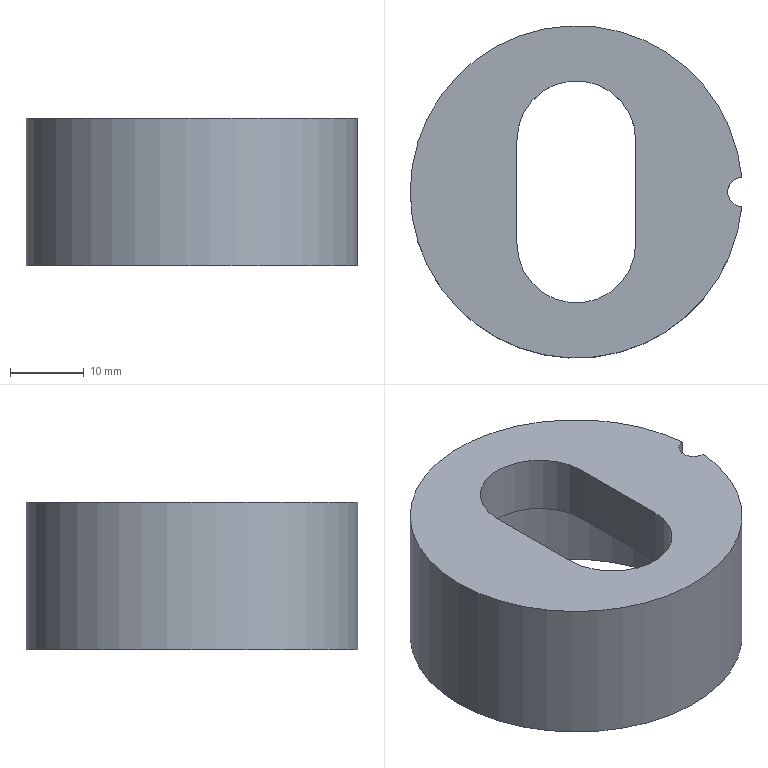Part | NX | features solid 2 | 1 solid | 10 faces | box 44.911 x 45 x 20 mm | volume 16039 mm3 | cylinder 5 | plane 5 | commonest cylinder face diameters 16.1 x2 4 x1 36 x1 45 x1
STEP:
#1=CARTESIAN_POINT('',(334.41,166.18,-1.322));
#2=VERTEX_POINT('',#1);
#3=CARTESIAN_POINT('',(334.41,166.18,18.678));
#4=VERTEX_POINT('',#3);
#5=CARTESIAN_POINT('',(334.41,166.18,8.678));
#6=DIRECTION('',(0.,0.,1.));
#7=VECTOR('',#6,1000.);
#8=LINE('',#5,#7);
#9=EDGE_CURVE('',#2,#4,#8,.T.);
#10=ORIENTED_EDGE('',*,*,#9,.F.);
#11=CARTESIAN_POINT('',(334.41,162.184,-1.322));
#12=VERTEX_POINT('',#11);
#13=CARTESIAN_POINT('',(311.999,164.182,-1.322));
#14=DIRECTION('',(0.,0.,1.));
#15=DIRECTION('',(1.,0.,0.));
#16=AXIS2_PLACEMENT_3D('',#13,#14,#15);
#17=CIRCLE('',#16,22.5);
#18=EDGE_CURVE('',#2,#12,#17,.T.);
#19=ORIENTED_EDGE('',*,*,#18,.T.);
#20=CARTESIAN_POINT('',(334.41,162.184,18.678));
#21=VERTEX_POINT('',#20);
#22=CARTESIAN_POINT('',(334.41,162.184,8.678));
#23=DIRECTION('',(0.,0.,1.));
#24=VECTOR('',#23,1000.);
#25=LINE('',#22,#24);
#26=EDGE_CURVE('',#21,#12,#25,.F.);
#27=ORIENTED_EDGE('',*,*,#26,.F.);
#28=CARTESIAN_POINT('',(311.999,164.182,18.678));
#29=DIRECTION('',(0.,0.,1.));
#30=DIRECTION('',(1.,0.,0.));
#31=AXIS2_PLACEMENT_3D('',#28,#29,#30);
#32=CIRCLE('',#31,22.5);
#33=EDGE_CURVE('',#4,#21,#32,.T.);
#34=ORIENTED_EDGE('',*,*,#33,.F.);
#35=EDGE_LOOP('',(#10,#19,#27,#34));
#36=FACE_BOUND('',#35,.T.);
#37=CARTESIAN_POINT('',(311.999,164.182,-1.322));
#38=DIRECTION('',(0.,0.,1.));
#39=DIRECTION('',(1.,0.,0.));
#40=AXIS2_PLACEMENT_3D('',#37,#38,#39);
#41=CYLINDRICAL_SURFACE('',#40,22.5);
#42=ADVANCED_FACE('',(#36),#41,.T.);
#43=CARTESIAN_POINT('',(329.999,164.182,-1.322));
#44=VERTEX_POINT('',#43);
#45=CARTESIAN_POINT('',(311.999,164.182,-1.322));
#46=DIRECTION('',(0.,0.,1.));
#47=DIRECTION('',(1.,0.,0.));
#48=AXIS2_PLACEMENT_3D('',#45,#46,#47);
#49=CIRCLE('',#48,18.);
#50=EDGE_CURVE('',#44,#44,#49,.T.);
#51=ORIENTED_EDGE('',*,*,#50,.T.);
#52=EDGE_LOOP('',(#51));
#53=FACE_BOUND('',#52,.T.);
#54=ORIENTED_EDGE('',*,*,#18,.F.);
#55=CARTESIAN_POINT('',(334.499,164.182,-1.322));
#56=DIRECTION('',(0.,0.,1.));
#57=DIRECTION('',(1.,0.,0.));
#58=AXIS2_PLACEMENT_3D('',#55,#56,#57);
#59=CIRCLE('',#58,2.);
#60=EDGE_CURVE('',#2,#12,#59,.T.);
#61=ORIENTED_EDGE('',*,*,#60,.T.);
#62=EDGE_LOOP('',(#54,#61));
#63=FACE_BOUND('',#62,.T.);
#64=CARTESIAN_POINT('',(311.999,164.182,-1.322));
#65=DIRECTION('',(0.,0.,1.));
#66=DIRECTION('',(1.,0.,0.));
#67=AXIS2_PLACEMENT_3D('',#64,#65,#66);
#68=PLANE('',#67);
#69=ADVANCED_FACE('',(#53,#63),#68,.F.);
#70=CARTESIAN_POINT('',(303.949,171.182,18.678));
#71=VERTEX_POINT('',#70);
#72=CARTESIAN_POINT('',(303.949,157.182,18.678));
#73=VERTEX_POINT('',#72);
#74=CARTESIAN_POINT('',(303.949,171.182,18.678));
#75=DIRECTION('',(0.,-1.,0.));
#76=VECTOR('',#75,1000.);
#77=LINE('',#74,#76);
#78=EDGE_CURVE('',#71,#73,#77,.T.);
#79=ORIENTED_EDGE('',*,*,#78,.F.);
#80=CARTESIAN_POINT('',(320.049,171.182,18.678));
#81=VERTEX_POINT('',#80);
#82=CARTESIAN_POINT('',(311.999,171.182,18.678));
#83=DIRECTION('',(0.,0.,1.));
#84=DIRECTION('',(1.,0.,0.));
#85=AXIS2_PLACEMENT_3D('',#82,#83,#84);
#86=CIRCLE('',#85,8.05);
#87=EDGE_CURVE('',#81,#71,#86,.T.);
#88=ORIENTED_EDGE('',*,*,#87,.F.);
#89=CARTESIAN_POINT('',(320.049,157.182,18.678));
#90=VERTEX_POINT('',#89);
#91=CARTESIAN_POINT('',(320.049,171.182,18.678));
#92=DIRECTION('',(0.,-1.,0.));
#93=VECTOR('',#92,1000.);
#94=LINE('',#91,#93);
#95=EDGE_CURVE('',#81,#90,#94,.T.);
#96=ORIENTED_EDGE('',*,*,#95,.T.);
#97=CARTESIAN_POINT('',(311.999,157.182,18.678));
#98=DIRECTION('',(0.,0.,1.));
#99=DIRECTION('',(1.,0.,0.));
#100=AXIS2_PLACEMENT_3D('',#97,#98,#99);
#101=CIRCLE('',#100,8.05);
#102=EDGE_CURVE('',#73,#90,#101,.T.);
#103=ORIENTED_EDGE('',*,*,#102,.F.);
#104=EDGE_LOOP('',(#79,#88,#96,#103));
#105=FACE_BOUND('',#104,.T.);
#106=CARTESIAN_POINT('',(334.499,164.182,18.678));
#107=DIRECTION('',(0.,0.,1.));
#108=DIRECTION('',(1.,0.,0.));
#109=AXIS2_PLACEMENT_3D('',#106,#107,#108);
#110=CIRCLE('',#109,2.);
#111=EDGE_CURVE('',#4,#21,#110,.T.);
#112=ORIENTED_EDGE('',*,*,#111,.F.);
#113=ORIENTED_EDGE('',*,*,#33,.T.);
#114=EDGE_LOOP('',(#112,#113));
#115=FACE_BOUND('',#114,.T.);
#116=CARTESIAN_POINT('',(311.999,164.182,18.678));
#117=DIRECTION('',(0.,0.,1.));
#118=DIRECTION('',(1.,0.,0.));
#119=AXIS2_PLACEMENT_3D('',#116,#117,#118);
#120=PLANE('',#119);
#121=ADVANCED_FACE('',(#105,#115),#120,.T.);
#122=ORIENTED_EDGE('',*,*,#50,.F.);
#123=EDGE_LOOP('',(#122));
#124=FACE_BOUND('',#123,.T.);
#125=CARTESIAN_POINT('',(329.999,164.182,10.678));
#126=VERTEX_POINT('',#125);
#127=CARTESIAN_POINT('',(311.999,164.182,10.678));
#128=DIRECTION('',(0.,0.,1.));
#129=DIRECTION('',(1.,0.,0.));
#130=AXIS2_PLACEMENT_3D('',#127,#128,#129);
#131=CIRCLE('',#130,18.);
#132=EDGE_CURVE('',#126,#126,#131,.T.);
#133=ORIENTED_EDGE('',*,*,#132,.T.);
#134=EDGE_LOOP('',(#133));
#135=FACE_BOUND('',#134,.T.);
#136=CARTESIAN_POINT('',(311.999,164.182,-1.322));
#137=DIRECTION('',(0.,0.,1.));
#138=DIRECTION('',(1.,0.,0.));
#139=AXIS2_PLACEMENT_3D('',#136,#137,#138);
#140=CYLINDRICAL_SURFACE('',#139,18.);
#141=ADVANCED_FACE('',(#124,#135),#140,.F.);
#142=CARTESIAN_POINT('',(320.049,171.182,10.678));
#143=VERTEX_POINT('',#142);
#144=CARTESIAN_POINT('',(303.949,171.182,10.678));
#145=VERTEX_POINT('',#144);
#146=CARTESIAN_POINT('',(311.999,171.182,10.678));
#147=DIRECTION('',(0.,0.,1.));
#148=DIRECTION('',(1.,0.,0.));
#149=AXIS2_PLACEMENT_3D('',#146,#147,#148);
#150=CIRCLE('',#149,8.05);
#151=EDGE_CURVE('',#143,#145,#150,.T.);
#152=ORIENTED_EDGE('',*,*,#151,.T.);
#153=CARTESIAN_POINT('',(303.949,157.182,10.678));
#154=VERTEX_POINT('',#153);
#155=CARTESIAN_POINT('',(303.949,164.182,10.678));
#156=DIRECTION('',(0.,-1.,0.));
#157=VECTOR('',#156,1000.);
#158=LINE('',#155,#157);
#159=EDGE_CURVE('',#145,#154,#158,.T.);
#160=ORIENTED_EDGE('',*,*,#159,.T.);
#161=CARTESIAN_POINT('',(320.049,157.182,10.678));
#162=VERTEX_POINT('',#161);
#163=CARTESIAN_POINT('',(311.999,157.182,10.678));
#164=DIRECTION('',(0.,0.,1.));
#165=DIRECTION('',(1.,0.,0.));
#166=AXIS2_PLACEMENT_3D('',#163,#164,#165);
#167=CIRCLE('',#166,8.05);
#168=EDGE_CURVE('',#154,#162,#167,.T.);
#169=ORIENTED_EDGE('',*,*,#168,.T.);
#170=CARTESIAN_POINT('',(320.049,164.182,10.678));
#171=DIRECTION('',(0.,-1.,0.));
#172=VECTOR('',#171,1000.);
#173=LINE('',#170,#172);
#174=EDGE_CURVE('',#143,#162,#173,.T.);
#175=ORIENTED_EDGE('',*,*,#174,.F.);
#176=EDGE_LOOP('',(#152,#160,#169,#175));
#177=FACE_BOUND('',#176,.T.);
#178=ORIENTED_EDGE('',*,*,#132,.F.);
#179=EDGE_LOOP('',(#178));
#180=FACE_BOUND('',#179,.T.);
#181=CARTESIAN_POINT('',(311.999,164.182,10.678));
#182=DIRECTION('',(0.,0.,1.));
#183=DIRECTION('',(1.,0.,0.));
#184=AXIS2_PLACEMENT_3D('',#181,#182,#183);
#185=PLANE('',#184);
#186=ADVANCED_FACE('',(#177,#180),#185,.F.);
#187=ORIENTED_EDGE('',*,*,#9,.T.);
#188=ORIENTED_EDGE('',*,*,#111,.T.);
#189=ORIENTED_EDGE('',*,*,#26,.T.);
#190=ORIENTED_EDGE('',*,*,#60,.F.);
#191=EDGE_LOOP('',(#187,#188,#189,#190));
#192=FACE_BOUND('',#191,.T.);
#193=CARTESIAN_POINT('',(334.499,164.182,-1.322));
#194=DIRECTION('',(0.,0.,1.));
#195=DIRECTION('',(1.,0.,0.));
#196=AXIS2_PLACEMENT_3D('',#193,#194,#195);
#197=CYLINDRICAL_SURFACE('',#196,2.);
#198=ADVANCED_FACE('',(#192),#197,.F.);
#199=CARTESIAN_POINT('',(303.949,171.182,-1.322));
#200=DIRECTION('',(0.,0.,1.));
#201=VECTOR('',#200,1000.);
#202=LINE('',#199,#201);
#203=EDGE_CURVE('',#145,#71,#202,.T.);
#204=ORIENTED_EDGE('',*,*,#203,.T.);
#205=ORIENTED_EDGE('',*,*,#78,.T.);
#206=CARTESIAN_POINT('',(303.949,157.182,-1.322));
#207=DIRECTION('',(0.,0.,1.));
#208=VECTOR('',#207,1000.);
#209=LINE('',#206,#208);
#210=EDGE_CURVE('',#154,#73,#209,.T.);
#211=ORIENTED_EDGE('',*,*,#210,.F.);
#212=ORIENTED_EDGE('',*,*,#159,.F.);
#213=EDGE_LOOP('',(#204,#205,#211,#212));
#214=FACE_BOUND('',#213,.T.);
#215=CARTESIAN_POINT('',(303.949,171.182,-1.322));
#216=DIRECTION('',(-1.,0.,0.));
#217=DIRECTION('',(0.,0.,1.));
#218=AXIS2_PLACEMENT_3D('',#215,#216,#217);
#219=PLANE('',#218);
#220=ADVANCED_FACE('',(#214),#219,.F.);
#221=ORIENTED_EDGE('',*,*,#210,.T.);
#222=ORIENTED_EDGE('',*,*,#102,.T.);
#223=CARTESIAN_POINT('',(320.049,157.182,-1.322));
#224=DIRECTION('',(0.,0.,1.));
#225=VECTOR('',#224,1000.);
#226=LINE('',#223,#225);
#227=EDGE_CURVE('',#162,#90,#226,.T.);
#228=ORIENTED_EDGE('',*,*,#227,.F.);
#229=ORIENTED_EDGE('',*,*,#168,.F.);
#230=EDGE_LOOP('',(#221,#222,#228,#229));
#231=FACE_BOUND('',#230,.T.);
#232=CARTESIAN_POINT('',(311.999,157.182,-1.322));
#233=DIRECTION('',(0.,0.,1.));
#234=DIRECTION('',(1.,0.,0.));
#235=AXIS2_PLACEMENT_3D('',#232,#233,#234);
#236=CYLINDRICAL_SURFACE('',#235,8.05);
#237=ADVANCED_FACE('',(#231),#236,.F.);
#238=ORIENTED_EDGE('',*,*,#174,.T.);
#239=ORIENTED_EDGE('',*,*,#227,.T.);
#240=ORIENTED_EDGE('',*,*,#95,.F.);
#241=CARTESIAN_POINT('',(320.049,171.182,-1.322));
#242=DIRECTION('',(0.,0.,1.));
#243=VECTOR('',#242,1000.);
#244=LINE('',#241,#243);
#245=EDGE_CURVE('',#143,#81,#244,.T.);
#246=ORIENTED_EDGE('',*,*,#245,.F.);
#247=EDGE_LOOP('',(#238,#239,#240,#246));
#248=FACE_BOUND('',#247,.T.);
#249=CARTESIAN_POINT('',(320.049,171.182,-1.322));
#250=DIRECTION('',(-1.,0.,0.));
#251=DIRECTION('',(0.,0.,1.));
#252=AXIS2_PLACEMENT_3D('',#249,#250,#251);
#253=PLANE('',#252);
#254=ADVANCED_FACE('',(#248),#253,.T.);
#255=ORIENTED_EDGE('',*,*,#245,.T.);
#256=ORIENTED_EDGE('',*,*,#87,.T.);
#257=ORIENTED_EDGE('',*,*,#203,.F.);
#258=ORIENTED_EDGE('',*,*,#151,.F.);
#259=EDGE_LOOP('',(#255,#256,#257,#258));
#260=FACE_BOUND('',#259,.T.);
#261=CARTESIAN_POINT('',(311.999,171.182,-1.322));
#262=DIRECTION('',(0.,0.,1.));
#263=DIRECTION('',(1.,0.,0.));
#264=AXIS2_PLACEMENT_3D('',#261,#262,#263);
#265=CYLINDRICAL_SURFACE('',#264,8.05);
#266=ADVANCED_FACE('',(#260),#265,.F.);
#267=CLOSED_SHELL('',(#42,#69,#121,#141,#186,#198,#220,#237,#254,#266));
#268=MANIFOLD_SOLID_BREP('',#267);
#269=(LENGTH_UNIT()NAMED_UNIT(*)SI_UNIT(.MILLI.,.METRE.));
#270=UNCERTAINTY_MEASURE_WITH_UNIT(LENGTH_MEASURE(0.00001),#269,'','');
#271=(NAMED_UNIT(*)PLANE_ANGLE_UNIT()SI_UNIT($,.RADIAN.));
#272=(NAMED_UNIT(*)SI_UNIT($,.STERADIAN.)SOLID_ANGLE_UNIT());
#273=(GEOMETRIC_REPRESENTATION_CONTEXT(3)GLOBAL_UNCERTAINTY_ASSIGNED_CONTEXT((#270))GLOBAL_UNIT_ASSIGNED_CONTEXT((#269,#271,#272))REPRESENTATION_CONTEXT('',''));
#274=ADVANCED_BREP_SHAPE_REPRESENTATION('',(#268),#273);